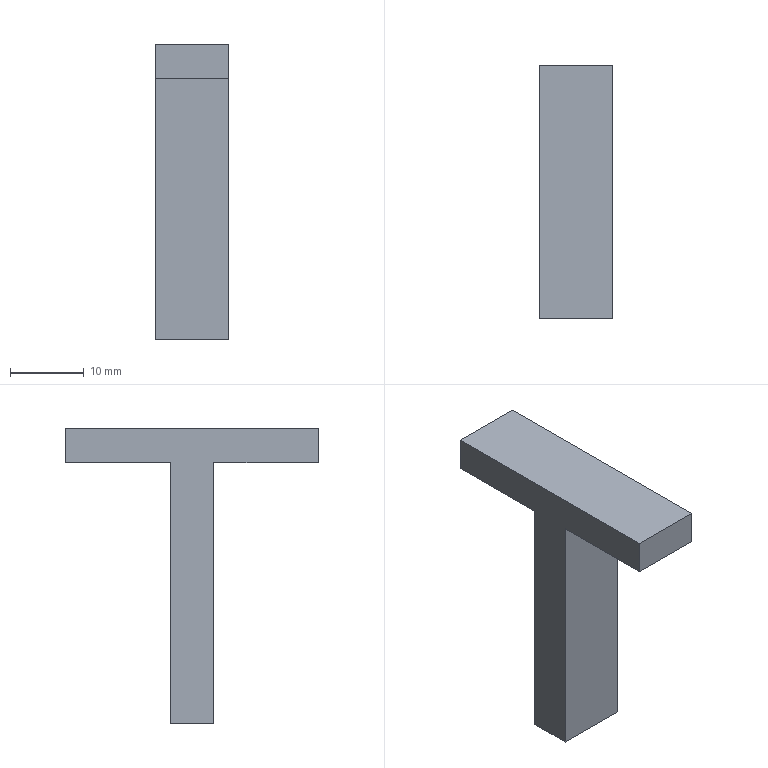Part | NX | features solid 2 | 1 solid | 10 faces | box 10 x 34.294 x 40 mm | volume 3670 mm3 | plane 10
STEP:
#1=CARTESIAN_POINT('',(2250.,339.869,-670.));
#2=VERTEX_POINT('',#1);
#3=CARTESIAN_POINT('',(2250.,334.01,-670.));
#4=VERTEX_POINT('',#3);
#5=CARTESIAN_POINT('',(2250.,339.869,-670.));
#6=CARTESIAN_POINT('',(2250.,337.916,-670.));
#7=CARTESIAN_POINT('',(2250.,335.963,-670.));
#8=CARTESIAN_POINT('',(2250.,334.01,-670.));
#9=B_SPLINE_CURVE_WITH_KNOTS('',3,(#5,#6,#7,#8),.UNSPECIFIED.,.F.,.F.,(4,4),(0.,0.03943),.PIECEWISE_BEZIER_KNOTS.);
#10=EDGE_CURVE('',#2,#4,#9,.T.);
#11=ORIENTED_EDGE('',*,*,#10,.F.);
#12=CARTESIAN_POINT('',(2260.,339.869,-670.));
#13=VERTEX_POINT('',#12);
#14=CARTESIAN_POINT('',(2260.,339.869,-670.));
#15=DIRECTION('',(-1.,0.,0.));
#16=VECTOR('',#15,1000.);
#17=LINE('',#14,#16);
#18=EDGE_CURVE('',#13,#2,#17,.T.);
#19=ORIENTED_EDGE('',*,*,#18,.F.);
#20=CARTESIAN_POINT('',(2260.,334.01,-670.));
#21=VERTEX_POINT('',#20);
#22=CARTESIAN_POINT('',(2260.,339.869,-670.));
#23=CARTESIAN_POINT('',(2260.,337.916,-670.));
#24=CARTESIAN_POINT('',(2260.,335.963,-670.));
#25=CARTESIAN_POINT('',(2260.,334.01,-670.));
#26=B_SPLINE_CURVE_WITH_KNOTS('',3,(#22,#23,#24,#25),.UNSPECIFIED.,.F.,.F.,(4,4),(0.,0.03943),.PIECEWISE_BEZIER_KNOTS.);
#27=EDGE_CURVE('',#13,#21,#26,.T.);
#28=ORIENTED_EDGE('',*,*,#27,.T.);
#29=CARTESIAN_POINT('',(2260.,334.01,-670.));
#30=DIRECTION('',(-1.,0.,0.));
#31=VECTOR('',#30,1000.);
#32=LINE('',#29,#31);
#33=EDGE_CURVE('',#21,#4,#32,.T.);
#34=ORIENTED_EDGE('',*,*,#33,.T.);
#35=EDGE_LOOP('',(#11,#19,#28,#34));
#36=FACE_BOUND('',#35,.T.);
#37=CARTESIAN_POINT('',(2260.,339.869,-670.));
#38=DIRECTION('',(0.,0.,-1.));
#39=DIRECTION('',(-1.,0.,0.));
#40=AXIS2_PLACEMENT_3D('',#37,#38,#39);
#41=PLANE('',#40);
#42=ADVANCED_FACE('',(#36),#41,.T.);
#43=CARTESIAN_POINT('',(2250.,334.01,-634.665));
#44=VERTEX_POINT('',#43);
#45=CARTESIAN_POINT('',(2250.,334.01,-670.));
#46=CARTESIAN_POINT('',(2250.,334.01,-658.222));
#47=CARTESIAN_POINT('',(2250.,334.01,-646.444));
#48=CARTESIAN_POINT('',(2250.,334.01,-634.665));
#49=B_SPLINE_CURVE_WITH_KNOTS('',3,(#45,#46,#47,#48),.UNSPECIFIED.,.F.,.F.,(4,4),(0.03943,0.2772),.PIECEWISE_BEZIER_KNOTS.);
#50=EDGE_CURVE('',#4,#44,#49,.T.);
#51=ORIENTED_EDGE('',*,*,#50,.F.);
#52=ORIENTED_EDGE('',*,*,#33,.F.);
#53=CARTESIAN_POINT('',(2260.,334.01,-634.665));
#54=VERTEX_POINT('',#53);
#55=CARTESIAN_POINT('',(2260.,334.01,-670.));
#56=CARTESIAN_POINT('',(2260.,334.01,-658.222));
#57=CARTESIAN_POINT('',(2260.,334.01,-646.444));
#58=CARTESIAN_POINT('',(2260.,334.01,-634.665));
#59=B_SPLINE_CURVE_WITH_KNOTS('',3,(#55,#56,#57,#58),.UNSPECIFIED.,.F.,.F.,(4,4),(0.03943,0.2772),.PIECEWISE_BEZIER_KNOTS.);
#60=EDGE_CURVE('',#21,#54,#59,.T.);
#61=ORIENTED_EDGE('',*,*,#60,.T.);
#62=CARTESIAN_POINT('',(2260.,334.01,-634.665));
#63=DIRECTION('',(-1.,0.,0.));
#64=VECTOR('',#63,1000.);
#65=LINE('',#62,#64);
#66=EDGE_CURVE('',#54,#44,#65,.T.);
#67=ORIENTED_EDGE('',*,*,#66,.T.);
#68=EDGE_LOOP('',(#51,#52,#61,#67));
#69=FACE_BOUND('',#68,.T.);
#70=CARTESIAN_POINT('',(2260.,334.01,-670.));
#71=DIRECTION('',(0.,-1.,0.));
#72=DIRECTION('',(1.,0.,0.));
#73=AXIS2_PLACEMENT_3D('',#70,#71,#72);
#74=PLANE('',#73);
#75=ADVANCED_FACE('',(#69),#74,.T.);
#76=CARTESIAN_POINT('',(2250.,319.8,-634.665));
#77=VERTEX_POINT('',#76);
#78=CARTESIAN_POINT('',(2250.,334.01,-634.665));
#79=CARTESIAN_POINT('',(2250.,329.274,-634.665));
#80=CARTESIAN_POINT('',(2250.,324.537,-634.665));
#81=CARTESIAN_POINT('',(2250.,319.8,-634.665));
#82=B_SPLINE_CURVE_WITH_KNOTS('',3,(#78,#79,#80,#81),.UNSPECIFIED.,.F.,.F.,(4,4),(0.2772,0.3729),.PIECEWISE_BEZIER_KNOTS.);
#83=EDGE_CURVE('',#44,#77,#82,.T.);
#84=ORIENTED_EDGE('',*,*,#83,.F.);
#85=ORIENTED_EDGE('',*,*,#66,.F.);
#86=CARTESIAN_POINT('',(2260.,319.8,-634.665));
#87=VERTEX_POINT('',#86);
#88=CARTESIAN_POINT('',(2260.,334.01,-634.665));
#89=CARTESIAN_POINT('',(2260.,329.274,-634.665));
#90=CARTESIAN_POINT('',(2260.,324.537,-634.665));
#91=CARTESIAN_POINT('',(2260.,319.8,-634.665));
#92=B_SPLINE_CURVE_WITH_KNOTS('',3,(#88,#89,#90,#91),.UNSPECIFIED.,.F.,.F.,(4,4),(0.2772,0.3729),.PIECEWISE_BEZIER_KNOTS.);
#93=EDGE_CURVE('',#54,#87,#92,.T.);
#94=ORIENTED_EDGE('',*,*,#93,.T.);
#95=CARTESIAN_POINT('',(2260.,319.8,-634.665));
#96=DIRECTION('',(-1.,0.,0.));
#97=VECTOR('',#96,1000.);
#98=LINE('',#95,#97);
#99=EDGE_CURVE('',#87,#77,#98,.T.);
#100=ORIENTED_EDGE('',*,*,#99,.T.);
#101=EDGE_LOOP('',(#84,#85,#94,#100));
#102=FACE_BOUND('',#101,.T.);
#103=CARTESIAN_POINT('',(2260.,334.01,-634.665));
#104=DIRECTION('',(0.,0.,-1.));
#105=DIRECTION('',(-1.,0.,0.));
#106=AXIS2_PLACEMENT_3D('',#103,#104,#105);
#107=PLANE('',#106);
#108=ADVANCED_FACE('',(#102),#107,.T.);
#109=CARTESIAN_POINT('',(2250.,319.8,-630.));
#110=VERTEX_POINT('',#109);
#111=CARTESIAN_POINT('',(2250.,319.8,-634.665));
#112=CARTESIAN_POINT('',(2250.,319.8,-633.11));
#113=CARTESIAN_POINT('',(2250.,319.8,-631.555));
#114=CARTESIAN_POINT('',(2250.,319.8,-630.));
#115=B_SPLINE_CURVE_WITH_KNOTS('',3,(#111,#112,#113,#114),.UNSPECIFIED.,.F.,.F.,(4,4),(0.3729,0.4043),.PIECEWISE_BEZIER_KNOTS.);
#116=EDGE_CURVE('',#77,#110,#115,.T.);
#117=ORIENTED_EDGE('',*,*,#116,.F.);
#118=ORIENTED_EDGE('',*,*,#99,.F.);
#119=CARTESIAN_POINT('',(2260.,319.8,-630.));
#120=VERTEX_POINT('',#119);
#121=CARTESIAN_POINT('',(2260.,319.8,-634.665));
#122=CARTESIAN_POINT('',(2260.,319.8,-633.11));
#123=CARTESIAN_POINT('',(2260.,319.8,-631.555));
#124=CARTESIAN_POINT('',(2260.,319.8,-630.));
#125=B_SPLINE_CURVE_WITH_KNOTS('',3,(#121,#122,#123,#124),.UNSPECIFIED.,.F.,.F.,(4,4),(0.3729,0.4043),.PIECEWISE_BEZIER_KNOTS.);
#126=EDGE_CURVE('',#87,#120,#125,.T.);
#127=ORIENTED_EDGE('',*,*,#126,.T.);
#128=CARTESIAN_POINT('',(2260.,319.8,-630.));
#129=DIRECTION('',(-1.,0.,0.));
#130=VECTOR('',#129,1000.);
#131=LINE('',#128,#130);
#132=EDGE_CURVE('',#120,#110,#131,.T.);
#133=ORIENTED_EDGE('',*,*,#132,.T.);
#134=EDGE_LOOP('',(#117,#118,#127,#133));
#135=FACE_BOUND('',#134,.T.);
#136=CARTESIAN_POINT('',(2260.,319.8,-634.665));
#137=DIRECTION('',(0.,-1.,0.));
#138=DIRECTION('',(1.,0.,0.));
#139=AXIS2_PLACEMENT_3D('',#136,#137,#138);
#140=PLANE('',#139);
#141=ADVANCED_FACE('',(#135),#140,.T.);
#142=CARTESIAN_POINT('',(2250.,354.094,-630.));
#143=VERTEX_POINT('',#142);
#144=CARTESIAN_POINT('',(2250.,319.8,-630.));
#145=CARTESIAN_POINT('',(2250.,331.231,-630.));
#146=CARTESIAN_POINT('',(2250.,342.663,-630.));
#147=CARTESIAN_POINT('',(2250.,354.094,-630.));
#148=B_SPLINE_CURVE_WITH_KNOTS('',3,(#144,#145,#146,#147),.UNSPECIFIED.,.F.,.F.,(4,4),(0.4043,0.6351),.PIECEWISE_BEZIER_KNOTS.);
#149=EDGE_CURVE('',#110,#143,#148,.T.);
#150=ORIENTED_EDGE('',*,*,#149,.F.);
#151=ORIENTED_EDGE('',*,*,#132,.F.);
#152=CARTESIAN_POINT('',(2260.,354.094,-630.));
#153=VERTEX_POINT('',#152);
#154=CARTESIAN_POINT('',(2260.,319.8,-630.));
#155=CARTESIAN_POINT('',(2260.,331.231,-630.));
#156=CARTESIAN_POINT('',(2260.,342.663,-630.));
#157=CARTESIAN_POINT('',(2260.,354.094,-630.));
#158=B_SPLINE_CURVE_WITH_KNOTS('',3,(#154,#155,#156,#157),.UNSPECIFIED.,.F.,.F.,(4,4),(0.4043,0.6351),.PIECEWISE_BEZIER_KNOTS.);
#159=EDGE_CURVE('',#120,#153,#158,.T.);
#160=ORIENTED_EDGE('',*,*,#159,.T.);
#161=CARTESIAN_POINT('',(2260.,354.094,-630.));
#162=DIRECTION('',(-1.,0.,0.));
#163=VECTOR('',#162,1000.);
#164=LINE('',#161,#163);
#165=EDGE_CURVE('',#153,#143,#164,.T.);
#166=ORIENTED_EDGE('',*,*,#165,.T.);
#167=EDGE_LOOP('',(#150,#151,#160,#166));
#168=FACE_BOUND('',#167,.T.);
#169=CARTESIAN_POINT('',(2260.,319.8,-630.));
#170=DIRECTION('',(0.,0.,1.));
#171=DIRECTION('',(1.,0.,0.));
#172=AXIS2_PLACEMENT_3D('',#169,#170,#171);
#173=PLANE('',#172);
#174=ADVANCED_FACE('',(#168),#173,.T.);
#175=CARTESIAN_POINT('',(2250.,354.094,-634.665));
#176=VERTEX_POINT('',#175);
#177=CARTESIAN_POINT('',(2250.,354.094,-630.));
#178=CARTESIAN_POINT('',(2250.,354.094,-631.555));
#179=CARTESIAN_POINT('',(2250.,354.094,-633.11));
#180=CARTESIAN_POINT('',(2250.,354.094,-634.665));
#181=B_SPLINE_CURVE_WITH_KNOTS('',3,(#177,#178,#179,#180),.UNSPECIFIED.,.F.,.F.,(4,4),(0.6351,0.6665),.PIECEWISE_BEZIER_KNOTS.);
#182=EDGE_CURVE('',#143,#176,#181,.T.);
#183=ORIENTED_EDGE('',*,*,#182,.F.);
#184=ORIENTED_EDGE('',*,*,#165,.F.);
#185=CARTESIAN_POINT('',(2260.,354.094,-634.665));
#186=VERTEX_POINT('',#185);
#187=CARTESIAN_POINT('',(2260.,354.094,-630.));
#188=CARTESIAN_POINT('',(2260.,354.094,-631.555));
#189=CARTESIAN_POINT('',(2260.,354.094,-633.11));
#190=CARTESIAN_POINT('',(2260.,354.094,-634.665));
#191=B_SPLINE_CURVE_WITH_KNOTS('',3,(#187,#188,#189,#190),.UNSPECIFIED.,.F.,.F.,(4,4),(0.6351,0.6665),.PIECEWISE_BEZIER_KNOTS.);
#192=EDGE_CURVE('',#153,#186,#191,.T.);
#193=ORIENTED_EDGE('',*,*,#192,.T.);
#194=CARTESIAN_POINT('',(2260.,354.094,-634.665));
#195=DIRECTION('',(-1.,0.,0.));
#196=VECTOR('',#195,1000.);
#197=LINE('',#194,#196);
#198=EDGE_CURVE('',#186,#176,#197,.T.);
#199=ORIENTED_EDGE('',*,*,#198,.T.);
#200=EDGE_LOOP('',(#183,#184,#193,#199));
#201=FACE_BOUND('',#200,.T.);
#202=CARTESIAN_POINT('',(2260.,354.094,-630.));
#203=DIRECTION('',(0.,1.,0.));
#204=DIRECTION('',(-1.,0.,0.));
#205=AXIS2_PLACEMENT_3D('',#202,#203,#204);
#206=PLANE('',#205);
#207=ADVANCED_FACE('',(#201),#206,.T.);
#208=CARTESIAN_POINT('',(2250.,339.869,-634.665));
#209=VERTEX_POINT('',#208);
#210=CARTESIAN_POINT('',(2250.,354.094,-634.665));
#211=CARTESIAN_POINT('',(2250.,349.353,-634.665));
#212=CARTESIAN_POINT('',(2250.,344.611,-634.665));
#213=CARTESIAN_POINT('',(2250.,339.869,-634.665));
#214=B_SPLINE_CURVE_WITH_KNOTS('',3,(#210,#211,#212,#213),.UNSPECIFIED.,.F.,.F.,(4,4),(0.6665,0.7622),.PIECEWISE_BEZIER_KNOTS.);
#215=EDGE_CURVE('',#176,#209,#214,.T.);
#216=ORIENTED_EDGE('',*,*,#215,.F.);
#217=ORIENTED_EDGE('',*,*,#198,.F.);
#218=CARTESIAN_POINT('',(2260.,339.869,-634.665));
#219=VERTEX_POINT('',#218);
#220=CARTESIAN_POINT('',(2260.,354.094,-634.665));
#221=CARTESIAN_POINT('',(2260.,349.353,-634.665));
#222=CARTESIAN_POINT('',(2260.,344.611,-634.665));
#223=CARTESIAN_POINT('',(2260.,339.869,-634.665));
#224=B_SPLINE_CURVE_WITH_KNOTS('',3,(#220,#221,#222,#223),.UNSPECIFIED.,.F.,.F.,(4,4),(0.6665,0.7622),.PIECEWISE_BEZIER_KNOTS.);
#225=EDGE_CURVE('',#186,#219,#224,.T.);
#226=ORIENTED_EDGE('',*,*,#225,.T.);
#227=CARTESIAN_POINT('',(2260.,339.869,-634.665));
#228=DIRECTION('',(-1.,0.,0.));
#229=VECTOR('',#228,1000.);
#230=LINE('',#227,#229);
#231=EDGE_CURVE('',#219,#209,#230,.T.);
#232=ORIENTED_EDGE('',*,*,#231,.T.);
#233=EDGE_LOOP('',(#216,#217,#226,#232));
#234=FACE_BOUND('',#233,.T.);
#235=CARTESIAN_POINT('',(2260.,354.094,-634.665));
#236=DIRECTION('',(0.,0.,-1.));
#237=DIRECTION('',(-1.,0.,0.));
#238=AXIS2_PLACEMENT_3D('',#235,#236,#237);
#239=PLANE('',#238);
#240=ADVANCED_FACE('',(#234),#239,.T.);
#241=CARTESIAN_POINT('',(2250.,339.869,-634.665));
#242=CARTESIAN_POINT('',(2250.,339.869,-646.444));
#243=CARTESIAN_POINT('',(2250.,339.869,-658.222));
#244=CARTESIAN_POINT('',(2250.,339.869,-670.));
#245=B_SPLINE_CURVE_WITH_KNOTS('',3,(#241,#242,#243,#244),.UNSPECIFIED.,.F.,.F.,(4,4),(0.7622,1.),.PIECEWISE_BEZIER_KNOTS.);
#246=EDGE_CURVE('',#209,#2,#245,.T.);
#247=ORIENTED_EDGE('',*,*,#246,.F.);
#248=ORIENTED_EDGE('',*,*,#231,.F.);
#249=CARTESIAN_POINT('',(2260.,339.869,-634.665));
#250=CARTESIAN_POINT('',(2260.,339.869,-646.444));
#251=CARTESIAN_POINT('',(2260.,339.869,-658.222));
#252=CARTESIAN_POINT('',(2260.,339.869,-670.));
#253=B_SPLINE_CURVE_WITH_KNOTS('',3,(#249,#250,#251,#252),.UNSPECIFIED.,.F.,.F.,(4,4),(0.7622,1.),.PIECEWISE_BEZIER_KNOTS.);
#254=EDGE_CURVE('',#219,#13,#253,.T.);
#255=ORIENTED_EDGE('',*,*,#254,.T.);
#256=ORIENTED_EDGE('',*,*,#18,.T.);
#257=EDGE_LOOP('',(#247,#248,#255,#256));
#258=FACE_BOUND('',#257,.T.);
#259=CARTESIAN_POINT('',(2260.,339.869,-634.665));
#260=DIRECTION('',(0.,1.,0.));
#261=DIRECTION('',(-1.,0.,0.));
#262=AXIS2_PLACEMENT_3D('',#259,#260,#261);
#263=PLANE('',#262);
#264=ADVANCED_FACE('',(#258),#263,.T.);
#265=ORIENTED_EDGE('',*,*,#27,.F.);
#266=ORIENTED_EDGE('',*,*,#254,.F.);
#267=ORIENTED_EDGE('',*,*,#225,.F.);
#268=ORIENTED_EDGE('',*,*,#192,.F.);
#269=ORIENTED_EDGE('',*,*,#159,.F.);
#270=ORIENTED_EDGE('',*,*,#126,.F.);
#271=ORIENTED_EDGE('',*,*,#93,.F.);
#272=ORIENTED_EDGE('',*,*,#60,.F.);
#273=EDGE_LOOP('',(#265,#266,#267,#268,#269,#270,#271,#272));
#274=FACE_BOUND('',#273,.T.);
#275=CARTESIAN_POINT('',(2260.,336.94,-670.));
#276=DIRECTION('',(1.,0.,0.));
#277=DIRECTION('',(0.,1.,0.));
#278=AXIS2_PLACEMENT_3D('',#275,#276,#277);
#279=PLANE('',#278);
#280=ADVANCED_FACE('',(#274),#279,.T.);
#281=ORIENTED_EDGE('',*,*,#10,.T.);
#282=ORIENTED_EDGE('',*,*,#50,.T.);
#283=ORIENTED_EDGE('',*,*,#83,.T.);
#284=ORIENTED_EDGE('',*,*,#116,.T.);
#285=ORIENTED_EDGE('',*,*,#149,.T.);
#286=ORIENTED_EDGE('',*,*,#182,.T.);
#287=ORIENTED_EDGE('',*,*,#215,.T.);
#288=ORIENTED_EDGE('',*,*,#246,.T.);
#289=EDGE_LOOP('',(#281,#282,#283,#284,#285,#286,#287,#288));
#290=FACE_BOUND('',#289,.T.);
#291=CARTESIAN_POINT('',(2250.,336.94,-670.));
#292=DIRECTION('',(1.,0.,0.));
#293=DIRECTION('',(0.,1.,0.));
#294=AXIS2_PLACEMENT_3D('',#291,#292,#293);
#295=PLANE('',#294);
#296=ADVANCED_FACE('',(#290),#295,.F.);
#297=CLOSED_SHELL('',(#42,#75,#108,#141,#174,#207,#240,#264,#280,#296));
#298=MANIFOLD_SOLID_BREP('',#297);
#299=(LENGTH_UNIT()NAMED_UNIT(*)SI_UNIT(.MILLI.,.METRE.));
#300=UNCERTAINTY_MEASURE_WITH_UNIT(LENGTH_MEASURE(0.00001),#299,'','');
#301=(NAMED_UNIT(*)PLANE_ANGLE_UNIT()SI_UNIT($,.RADIAN.));
#302=(NAMED_UNIT(*)SI_UNIT($,.STERADIAN.)SOLID_ANGLE_UNIT());
#303=(GEOMETRIC_REPRESENTATION_CONTEXT(3)GLOBAL_UNCERTAINTY_ASSIGNED_CONTEXT((#300))GLOBAL_UNIT_ASSIGNED_CONTEXT((#299,#301,#302))REPRESENTATION_CONTEXT('',''));
#304=ADVANCED_BREP_SHAPE_REPRESENTATION('',(#298),#303);